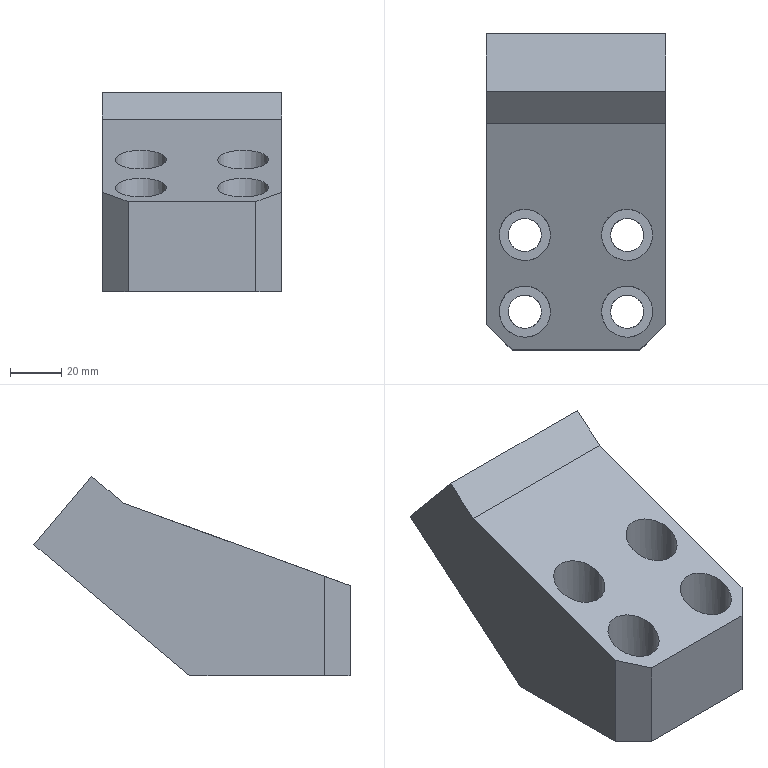Part | NX | features solid 2 | 1 solid | 22 faces | box 70 x 123.603 x 77.991 mm | volume 327595 mm3 | plane 14 | cylinder 8 | commonest cylinder face diameters 13 x4 20 x4
STEP:
#1=CARTESIAN_POINT('',(-535.,-473.5,-185.));
#2=VERTEX_POINT('',#1);
#3=CARTESIAN_POINT('',(-535.,-480.,-185.));
#4=DIRECTION('',(0.,0.,1.));
#5=DIRECTION('',(0.,1.,0.));
#6=AXIS2_PLACEMENT_3D('',#3,#4,#5);
#7=CIRCLE('',#6,6.5);
#8=EDGE_CURVE('',#2,#2,#7,.T.);
#9=ORIENTED_EDGE('',*,*,#8,.F.);
#10=EDGE_LOOP('',(#9));
#11=FACE_BOUND('',#10,.T.);
#12=CARTESIAN_POINT('',(-528.5,-480.,-165.));
#13=VERTEX_POINT('',#12);
#14=CARTESIAN_POINT('',(-535.,-480.,-165.));
#15=DIRECTION('',(0.,0.,1.));
#16=DIRECTION('',(1.,0.,0.));
#17=AXIS2_PLACEMENT_3D('',#14,#15,#16);
#18=CIRCLE('',#17,6.5);
#19=EDGE_CURVE('',#13,#13,#18,.F.);
#20=ORIENTED_EDGE('',*,*,#19,.F.);
#21=EDGE_LOOP('',(#20));
#22=FACE_BOUND('',#21,.T.);
#23=CARTESIAN_POINT('',(-535.,-480.,-135.));
#24=DIRECTION('',(0.,0.,-1.));
#25=DIRECTION('',(0.,-1.,0.));
#26=AXIS2_PLACEMENT_3D('',#23,#24,#25);
#27=CYLINDRICAL_SURFACE('',#26,6.5);
#28=ADVANCED_FACE('',(#11,#22),#27,.F.);
#29=CARTESIAN_POINT('',(-495.,-473.5,-185.));
#30=VERTEX_POINT('',#29);
#31=CARTESIAN_POINT('',(-495.,-480.,-185.));
#32=DIRECTION('',(0.,0.,1.));
#33=DIRECTION('',(0.,1.,0.));
#34=AXIS2_PLACEMENT_3D('',#31,#32,#33);
#35=CIRCLE('',#34,6.5);
#36=EDGE_CURVE('',#30,#30,#35,.T.);
#37=ORIENTED_EDGE('',*,*,#36,.F.);
#38=EDGE_LOOP('',(#37));
#39=FACE_BOUND('',#38,.T.);
#40=CARTESIAN_POINT('',(-488.5,-480.,-165.));
#41=VERTEX_POINT('',#40);
#42=CARTESIAN_POINT('',(-495.,-480.,-165.));
#43=DIRECTION('',(0.,0.,1.));
#44=DIRECTION('',(1.,0.,0.));
#45=AXIS2_PLACEMENT_3D('',#42,#43,#44);
#46=CIRCLE('',#45,6.5);
#47=EDGE_CURVE('',#41,#41,#46,.F.);
#48=ORIENTED_EDGE('',*,*,#47,.F.);
#49=EDGE_LOOP('',(#48));
#50=FACE_BOUND('',#49,.T.);
#51=CARTESIAN_POINT('',(-495.,-480.,-135.));
#52=DIRECTION('',(0.,0.,-1.));
#53=DIRECTION('',(0.,-1.,0.));
#54=AXIS2_PLACEMENT_3D('',#51,#52,#53);
#55=CYLINDRICAL_SURFACE('',#54,6.5);
#56=ADVANCED_FACE('',(#39,#50),#55,.F.);
#57=CARTESIAN_POINT('',(-495.,-503.5,-185.));
#58=VERTEX_POINT('',#57);
#59=CARTESIAN_POINT('',(-495.,-510.,-185.));
#60=DIRECTION('',(0.,0.,1.));
#61=DIRECTION('',(0.,1.,0.));
#62=AXIS2_PLACEMENT_3D('',#59,#60,#61);
#63=CIRCLE('',#62,6.5);
#64=EDGE_CURVE('',#58,#58,#63,.T.);
#65=ORIENTED_EDGE('',*,*,#64,.F.);
#66=EDGE_LOOP('',(#65));
#67=FACE_BOUND('',#66,.T.);
#68=CARTESIAN_POINT('',(-488.5,-510.,-165.));
#69=VERTEX_POINT('',#68);
#70=CARTESIAN_POINT('',(-495.,-510.,-165.));
#71=DIRECTION('',(0.,0.,1.));
#72=DIRECTION('',(1.,0.,0.));
#73=AXIS2_PLACEMENT_3D('',#70,#71,#72);
#74=CIRCLE('',#73,6.5);
#75=EDGE_CURVE('',#69,#69,#74,.F.);
#76=ORIENTED_EDGE('',*,*,#75,.F.);
#77=EDGE_LOOP('',(#76));
#78=FACE_BOUND('',#77,.T.);
#79=CARTESIAN_POINT('',(-495.,-510.,-135.));
#80=DIRECTION('',(0.,0.,-1.));
#81=DIRECTION('',(0.,-1.,0.));
#82=AXIS2_PLACEMENT_3D('',#79,#80,#81);
#83=CYLINDRICAL_SURFACE('',#82,6.5);
#84=ADVANCED_FACE('',(#67,#78),#83,.F.);
#85=CARTESIAN_POINT('',(-535.,-503.5,-185.));
#86=VERTEX_POINT('',#85);
#87=CARTESIAN_POINT('',(-535.,-510.,-185.));
#88=DIRECTION('',(0.,0.,1.));
#89=DIRECTION('',(0.,1.,0.));
#90=AXIS2_PLACEMENT_3D('',#87,#88,#89);
#91=CIRCLE('',#90,6.5);
#92=EDGE_CURVE('',#86,#86,#91,.T.);
#93=ORIENTED_EDGE('',*,*,#92,.F.);
#94=EDGE_LOOP('',(#93));
#95=FACE_BOUND('',#94,.T.);
#96=CARTESIAN_POINT('',(-528.5,-510.,-165.));
#97=VERTEX_POINT('',#96);
#98=CARTESIAN_POINT('',(-535.,-510.,-165.));
#99=DIRECTION('',(0.,0.,1.));
#100=DIRECTION('',(1.,0.,0.));
#101=AXIS2_PLACEMENT_3D('',#98,#99,#100);
#102=CIRCLE('',#101,6.5);
#103=EDGE_CURVE('',#97,#97,#102,.F.);
#104=ORIENTED_EDGE('',*,*,#103,.F.);
#105=EDGE_LOOP('',(#104));
#106=FACE_BOUND('',#105,.T.);
#107=CARTESIAN_POINT('',(-535.,-510.,-135.));
#108=DIRECTION('',(0.,0.,-1.));
#109=DIRECTION('',(0.,-1.,0.));
#110=AXIS2_PLACEMENT_3D('',#107,#108,#109);
#111=CYLINDRICAL_SURFACE('',#110,6.5);
#112=ADVANCED_FACE('',(#95,#106),#111,.F.);
#113=CARTESIAN_POINT('',(-540.,-525.,-185.));
#114=VERTEX_POINT('',#113);
#115=CARTESIAN_POINT('',(-490.,-525.,-185.));
#116=VERTEX_POINT('',#115);
#117=CARTESIAN_POINT('',(-535.,-525.,-185.));
#118=DIRECTION('',(-1.,0.,0.));
#119=VECTOR('',#118,1000.);
#120=LINE('',#117,#119);
#121=EDGE_CURVE('',#114,#116,#120,.F.);
#122=ORIENTED_EDGE('',*,*,#121,.T.);
#123=CARTESIAN_POINT('',(-490.,-525.,-149.753));
#124=VERTEX_POINT('',#123);
#125=CARTESIAN_POINT('',(-490.,-525.,-188.825));
#126=DIRECTION('',(0.,0.,-1.));
#127=VECTOR('',#126,1000.);
#128=LINE('',#125,#127);
#129=EDGE_CURVE('',#116,#124,#128,.F.);
#130=ORIENTED_EDGE('',*,*,#129,.T.);
#131=CARTESIAN_POINT('',(-540.,-525.,-149.753));
#132=VERTEX_POINT('',#131);
#133=CARTESIAN_POINT('',(-535.,-525.,-149.753));
#134=DIRECTION('',(1.,0.,0.));
#135=VECTOR('',#134,1000.);
#136=LINE('',#133,#135);
#137=EDGE_CURVE('',#124,#132,#136,.F.);
#138=ORIENTED_EDGE('',*,*,#137,.T.);
#139=CARTESIAN_POINT('',(-540.,-525.,-188.825));
#140=DIRECTION('',(0.,0.,1.));
#141=VECTOR('',#140,1000.);
#142=LINE('',#139,#141);
#143=EDGE_CURVE('',#132,#114,#142,.F.);
#144=ORIENTED_EDGE('',*,*,#143,.T.);
#145=EDGE_LOOP('',(#122,#130,#138,#144));
#146=FACE_BOUND('',#145,.T.);
#147=CARTESIAN_POINT('',(-535.,-525.,-188.825));
#148=DIRECTION('',(0.,-1.,0.));
#149=DIRECTION('',(1.,0.,0.));
#150=AXIS2_PLACEMENT_3D('',#147,#148,#149);
#151=PLANE('',#150);
#152=ADVANCED_FACE('',(#146),#151,.T.);
#153=CARTESIAN_POINT('',(-480.,-515.,-146.113));
#154=VERTEX_POINT('',#153);
#155=CARTESIAN_POINT('',(-480.,-515.,-185.));
#156=VERTEX_POINT('',#155);
#157=CARTESIAN_POINT('',(-480.,-515.,-188.825));
#158=DIRECTION('',(0.,0.,1.));
#159=VECTOR('',#158,1000.);
#160=LINE('',#157,#159);
#161=EDGE_CURVE('',#154,#156,#160,.F.);
#162=ORIENTED_EDGE('',*,*,#161,.T.);
#163=CARTESIAN_POINT('',(-480.,-462.389,-185.));
#164=VERTEX_POINT('',#163);
#165=CARTESIAN_POINT('',(-480.,-492.776,-185.));
#166=DIRECTION('',(0.,-1.,0.));
#167=VECTOR('',#166,1000.);
#168=LINE('',#165,#167);
#169=EDGE_CURVE('',#156,#164,#168,.F.);
#170=ORIENTED_EDGE('',*,*,#169,.T.);
#171=CARTESIAN_POINT('',(-480.,-401.397,-133.821));
#172=VERTEX_POINT('',#171);
#173=CARTESIAN_POINT('',(-480.,-482.104,-201.543));
#174=DIRECTION('',(0.,-0.766,-0.6428));
#175=VECTOR('',#174,1000.);
#176=LINE('',#173,#175);
#177=EDGE_CURVE('',#164,#172,#176,.F.);
#178=ORIENTED_EDGE('',*,*,#177,.T.);
#179=CARTESIAN_POINT('',(-480.,-423.894,-107.009));
#180=VERTEX_POINT('',#179);
#181=CARTESIAN_POINT('',(-480.,-406.76,-127.429));
#182=DIRECTION('',(0.,0.6428,-0.766));
#183=VECTOR('',#182,1000.);
#184=LINE('',#181,#183);
#185=EDGE_CURVE('',#180,#172,#184,.T.);
#186=ORIENTED_EDGE('',*,*,#185,.F.);
#187=CARTESIAN_POINT('',(-480.,-436.404,-117.506));
#188=VERTEX_POINT('',#187);
#189=CARTESIAN_POINT('',(-480.,-435.385,-116.651));
#190=DIRECTION('',(0.,-0.766,-0.6428));
#191=VECTOR('',#190,1000.);
#192=LINE('',#189,#191);
#193=EDGE_CURVE('',#188,#180,#192,.F.);
#194=ORIENTED_EDGE('',*,*,#193,.F.);
#195=CARTESIAN_POINT('',(-480.,-509.103,-143.966));
#196=DIRECTION('',(0.,0.9397,0.342));
#197=VECTOR('',#196,1000.);
#198=LINE('',#195,#197);
#199=EDGE_CURVE('',#154,#188,#198,.T.);
#200=ORIENTED_EDGE('',*,*,#199,.F.);
#201=EDGE_LOOP('',(#162,#170,#178,#186,#194,#200));
#202=FACE_BOUND('',#201,.T.);
#203=CARTESIAN_POINT('',(-480.,-492.776,-188.825));
#204=DIRECTION('',(1.,0.,0.));
#205=DIRECTION('',(0.,1.,0.));
#206=AXIS2_PLACEMENT_3D('',#203,#204,#205);
#207=PLANE('',#206);
#208=ADVANCED_FACE('',(#202),#207,.T.);
#209=CARTESIAN_POINT('',(-550.,-436.404,-117.506));
#210=VERTEX_POINT('',#209);
#211=CARTESIAN_POINT('',(-550.,-423.894,-107.009));
#212=VERTEX_POINT('',#211);
#213=CARTESIAN_POINT('',(-550.,-504.602,-174.731));
#214=DIRECTION('',(0.,0.766,0.6428));
#215=VECTOR('',#214,1000.);
#216=LINE('',#213,#215);
#217=EDGE_CURVE('',#210,#212,#216,.T.);
#218=ORIENTED_EDGE('',*,*,#217,.T.);
#219=CARTESIAN_POINT('',(-550.,-401.397,-133.821));
#220=VERTEX_POINT('',#219);
#221=CARTESIAN_POINT('',(-550.,-406.76,-127.429));
#222=DIRECTION('',(0.,-0.6428,0.766));
#223=VECTOR('',#222,1000.);
#224=LINE('',#221,#223);
#225=EDGE_CURVE('',#220,#212,#224,.T.);
#226=ORIENTED_EDGE('',*,*,#225,.F.);
#227=CARTESIAN_POINT('',(-550.,-462.389,-185.));
#228=VERTEX_POINT('',#227);
#229=CARTESIAN_POINT('',(-550.,-412.887,-143.463));
#230=DIRECTION('',(0.,0.766,0.6428));
#231=VECTOR('',#230,1000.);
#232=LINE('',#229,#231);
#233=EDGE_CURVE('',#228,#220,#232,.T.);
#234=ORIENTED_EDGE('',*,*,#233,.F.);
#235=CARTESIAN_POINT('',(-550.,-515.,-185.));
#236=VERTEX_POINT('',#235);
#237=CARTESIAN_POINT('',(-550.,-492.776,-185.));
#238=DIRECTION('',(0.,-1.,0.));
#239=VECTOR('',#238,1000.);
#240=LINE('',#237,#239);
#241=EDGE_CURVE('',#228,#236,#240,.T.);
#242=ORIENTED_EDGE('',*,*,#241,.T.);
#243=CARTESIAN_POINT('',(-550.,-515.,-146.113));
#244=VERTEX_POINT('',#243);
#245=CARTESIAN_POINT('',(-550.,-515.,-188.825));
#246=DIRECTION('',(0.,0.,1.));
#247=VECTOR('',#246,1000.);
#248=LINE('',#245,#247);
#249=EDGE_CURVE('',#236,#244,#248,.T.);
#250=ORIENTED_EDGE('',*,*,#249,.T.);
#251=CARTESIAN_POINT('',(-550.,-509.103,-143.966));
#252=DIRECTION('',(0.,0.9397,0.342));
#253=VECTOR('',#252,1000.);
#254=LINE('',#251,#253);
#255=EDGE_CURVE('',#210,#244,#254,.F.);
#256=ORIENTED_EDGE('',*,*,#255,.F.);
#257=EDGE_LOOP('',(#218,#226,#234,#242,#250,#256));
#258=FACE_BOUND('',#257,.T.);
#259=CARTESIAN_POINT('',(-550.,-492.776,-188.825));
#260=DIRECTION('',(1.,0.,0.));
#261=DIRECTION('',(0.,1.,0.));
#262=AXIS2_PLACEMENT_3D('',#259,#260,#261);
#263=PLANE('',#262);
#264=ADVANCED_FACE('',(#258),#263,.F.);
#265=ORIENTED_EDGE('',*,*,#64,.T.);
#266=EDGE_LOOP('',(#265));
#267=FACE_BOUND('',#266,.T.);
#268=ORIENTED_EDGE('',*,*,#92,.T.);
#269=EDGE_LOOP('',(#268));
#270=FACE_BOUND('',#269,.T.);
#271=ORIENTED_EDGE('',*,*,#169,.F.);
#272=CARTESIAN_POINT('',(-480.,-515.,-185.));
#273=DIRECTION('',(0.7071,0.7071,0.));
#274=VECTOR('',#273,1000.);
#275=LINE('',#272,#274);
#276=EDGE_CURVE('',#156,#116,#275,.F.);
#277=ORIENTED_EDGE('',*,*,#276,.T.);
#278=ORIENTED_EDGE('',*,*,#121,.F.);
#279=CARTESIAN_POINT('',(-540.,-525.,-185.));
#280=DIRECTION('',(-0.7071,0.7071,0.));
#281=VECTOR('',#280,1000.);
#282=LINE('',#279,#281);
#283=EDGE_CURVE('',#114,#236,#282,.T.);
#284=ORIENTED_EDGE('',*,*,#283,.T.);
#285=ORIENTED_EDGE('',*,*,#241,.F.);
#286=CARTESIAN_POINT('',(-515.,-462.389,-185.));
#287=DIRECTION('',(-1.,0.,0.));
#288=VECTOR('',#287,1000.);
#289=LINE('',#286,#288);
#290=EDGE_CURVE('',#164,#228,#289,.T.);
#291=ORIENTED_EDGE('',*,*,#290,.F.);
#292=EDGE_LOOP('',(#271,#277,#278,#284,#285,#291));
#293=FACE_BOUND('',#292,.T.);
#294=ORIENTED_EDGE('',*,*,#36,.T.);
#295=EDGE_LOOP('',(#294));
#296=FACE_BOUND('',#295,.T.);
#297=ORIENTED_EDGE('',*,*,#8,.T.);
#298=EDGE_LOOP('',(#297));
#299=FACE_BOUND('',#298,.T.);
#300=CARTESIAN_POINT('',(-203.,-82.,-185.));
#301=DIRECTION('',(0.,0.,1.));
#302=DIRECTION('',(0.,1.,0.));
#303=AXIS2_PLACEMENT_3D('',#300,#301,#302);
#304=PLANE('',#303);
#305=ADVANCED_FACE('',(#267,#270,#293,#296,#299),#304,.F.);
#306=ORIENTED_EDGE('',*,*,#129,.F.);
#307=ORIENTED_EDGE('',*,*,#276,.F.);
#308=ORIENTED_EDGE('',*,*,#161,.F.);
#309=CARTESIAN_POINT('',(-469.616,-504.616,-142.333));
#310=DIRECTION('',(0.6848,0.6848,0.2492));
#311=VECTOR('',#310,1000.);
#312=LINE('',#309,#311);
#313=EDGE_CURVE('',#124,#154,#312,.T.);
#314=ORIENTED_EDGE('',*,*,#313,.F.);
#315=EDGE_LOOP('',(#306,#307,#308,#314));
#316=FACE_BOUND('',#315,.T.);
#317=CARTESIAN_POINT('',(-480.,-515.,-188.825));
#318=DIRECTION('',(-0.7071,0.7071,0.));
#319=DIRECTION('',(-0.7071,-0.7071,0.));
#320=AXIS2_PLACEMENT_3D('',#317,#318,#319);
#321=PLANE('',#320);
#322=ADVANCED_FACE('',(#316),#321,.F.);
#323=CARTESIAN_POINT('',(-533.331,-531.669,-152.18));
#324=DIRECTION('',(0.6848,-0.6848,-0.2492));
#325=VECTOR('',#324,1000.);
#326=LINE('',#323,#325);
#327=EDGE_CURVE('',#132,#244,#326,.F.);
#328=ORIENTED_EDGE('',*,*,#327,.T.);
#329=ORIENTED_EDGE('',*,*,#249,.F.);
#330=ORIENTED_EDGE('',*,*,#283,.F.);
#331=ORIENTED_EDGE('',*,*,#143,.F.);
#332=EDGE_LOOP('',(#328,#329,#330,#331));
#333=FACE_BOUND('',#332,.T.);
#334=CARTESIAN_POINT('',(-540.,-525.,-188.825));
#335=DIRECTION('',(-0.7071,-0.7071,0.));
#336=DIRECTION('',(0.7071,-0.7071,0.));
#337=AXIS2_PLACEMENT_3D('',#334,#335,#336);
#338=PLANE('',#337);
#339=ADVANCED_FACE('',(#333),#338,.T.);
#340=CARTESIAN_POINT('',(-525.,-510.,-165.));
#341=VERTEX_POINT('',#340);
#342=CARTESIAN_POINT('',(-535.,-510.,-165.));
#343=DIRECTION('',(0.,0.,1.));
#344=DIRECTION('',(1.,0.,0.));
#345=AXIS2_PLACEMENT_3D('',#342,#343,#344);
#346=CIRCLE('',#345,10.);
#347=EDGE_CURVE('',#341,#341,#346,.T.);
#348=ORIENTED_EDGE('',*,*,#347,.T.);
#349=EDGE_LOOP('',(#348));
#350=FACE_BOUND('',#349,.T.);
#351=ORIENTED_EDGE('',*,*,#103,.T.);
#352=EDGE_LOOP('',(#351));
#353=FACE_BOUND('',#352,.T.);
#354=CARTESIAN_POINT('',(-535.,-510.,-165.));
#355=DIRECTION('',(0.,0.,1.));
#356=DIRECTION('',(0.,1.,0.));
#357=AXIS2_PLACEMENT_3D('',#354,#355,#356);
#358=PLANE('',#357);
#359=ADVANCED_FACE('',(#350,#353),#358,.T.);
#360=CARTESIAN_POINT('',(-535.,-520.,-147.933));
#361=VERTEX_POINT('',#360);
#362=CARTESIAN_POINT('',(-535.,-510.,-144.293));
#363=DIRECTION('',(0.,0.342,-0.9397));
#364=DIRECTION('',(0.,-0.9397,-0.342));
#365=AXIS2_PLACEMENT_3D('',#362,#363,#364);
#366=ELLIPSE('',#365,10.642,10.);
#367=EDGE_CURVE('',#361,#361,#366,.T.);
#368=ORIENTED_EDGE('',*,*,#367,.F.);
#369=EDGE_LOOP('',(#368));
#370=FACE_BOUND('',#369,.T.);
#371=ORIENTED_EDGE('',*,*,#347,.F.);
#372=EDGE_LOOP('',(#371));
#373=FACE_BOUND('',#372,.T.);
#374=CARTESIAN_POINT('',(-535.,-510.,15.));
#375=DIRECTION('',(0.,0.,-1.));
#376=DIRECTION('',(0.,-1.,0.));
#377=AXIS2_PLACEMENT_3D('',#374,#375,#376);
#378=CYLINDRICAL_SURFACE('',#377,10.);
#379=ADVANCED_FACE('',(#370,#373),#378,.F.);
#380=CARTESIAN_POINT('',(-485.,-510.,-165.));
#381=VERTEX_POINT('',#380);
#382=CARTESIAN_POINT('',(-495.,-510.,-165.));
#383=DIRECTION('',(0.,0.,1.));
#384=DIRECTION('',(1.,0.,0.));
#385=AXIS2_PLACEMENT_3D('',#382,#383,#384);
#386=CIRCLE('',#385,10.);
#387=EDGE_CURVE('',#381,#381,#386,.T.);
#388=ORIENTED_EDGE('',*,*,#387,.T.);
#389=EDGE_LOOP('',(#388));
#390=FACE_BOUND('',#389,.T.);
#391=ORIENTED_EDGE('',*,*,#75,.T.);
#392=EDGE_LOOP('',(#391));
#393=FACE_BOUND('',#392,.T.);
#394=CARTESIAN_POINT('',(-495.,-510.,-165.));
#395=DIRECTION('',(0.,0.,1.));
#396=DIRECTION('',(0.,1.,0.));
#397=AXIS2_PLACEMENT_3D('',#394,#395,#396);
#398=PLANE('',#397);
#399=ADVANCED_FACE('',(#390,#393),#398,.T.);
#400=CARTESIAN_POINT('',(-495.,-520.,-147.933));
#401=VERTEX_POINT('',#400);
#402=CARTESIAN_POINT('',(-495.,-510.,-144.293));
#403=DIRECTION('',(0.,0.342,-0.9397));
#404=DIRECTION('',(0.,-0.9397,-0.342));
#405=AXIS2_PLACEMENT_3D('',#402,#403,#404);
#406=ELLIPSE('',#405,10.642,10.);
#407=EDGE_CURVE('',#401,#401,#406,.T.);
#408=ORIENTED_EDGE('',*,*,#407,.F.);
#409=EDGE_LOOP('',(#408));
#410=FACE_BOUND('',#409,.T.);
#411=ORIENTED_EDGE('',*,*,#387,.F.);
#412=EDGE_LOOP('',(#411));
#413=FACE_BOUND('',#412,.T.);
#414=CARTESIAN_POINT('',(-495.,-510.,15.));
#415=DIRECTION('',(0.,0.,-1.));
#416=DIRECTION('',(0.,-1.,0.));
#417=AXIS2_PLACEMENT_3D('',#414,#415,#416);
#418=CYLINDRICAL_SURFACE('',#417,10.);
#419=ADVANCED_FACE('',(#410,#413),#418,.F.);
#420=CARTESIAN_POINT('',(-485.,-480.,-165.));
#421=VERTEX_POINT('',#420);
#422=CARTESIAN_POINT('',(-495.,-480.,-165.));
#423=DIRECTION('',(0.,0.,1.));
#424=DIRECTION('',(1.,0.,0.));
#425=AXIS2_PLACEMENT_3D('',#422,#423,#424);
#426=CIRCLE('',#425,10.);
#427=EDGE_CURVE('',#421,#421,#426,.T.);
#428=ORIENTED_EDGE('',*,*,#427,.T.);
#429=EDGE_LOOP('',(#428));
#430=FACE_BOUND('',#429,.T.);
#431=ORIENTED_EDGE('',*,*,#47,.T.);
#432=EDGE_LOOP('',(#431));
#433=FACE_BOUND('',#432,.T.);
#434=CARTESIAN_POINT('',(-495.,-480.,-165.));
#435=DIRECTION('',(0.,0.,1.));
#436=DIRECTION('',(0.,1.,0.));
#437=AXIS2_PLACEMENT_3D('',#434,#435,#436);
#438=PLANE('',#437);
#439=ADVANCED_FACE('',(#430,#433),#438,.T.);
#440=CARTESIAN_POINT('',(-495.,-490.,-137.014));
#441=VERTEX_POINT('',#440);
#442=CARTESIAN_POINT('',(-495.,-480.,-133.374));
#443=DIRECTION('',(0.,0.342,-0.9397));
#444=DIRECTION('',(0.,-0.9397,-0.342));
#445=AXIS2_PLACEMENT_3D('',#442,#443,#444);
#446=ELLIPSE('',#445,10.642,10.);
#447=EDGE_CURVE('',#441,#441,#446,.T.);
#448=ORIENTED_EDGE('',*,*,#447,.F.);
#449=EDGE_LOOP('',(#448));
#450=FACE_BOUND('',#449,.T.);
#451=ORIENTED_EDGE('',*,*,#427,.F.);
#452=EDGE_LOOP('',(#451));
#453=FACE_BOUND('',#452,.T.);
#454=CARTESIAN_POINT('',(-495.,-480.,15.));
#455=DIRECTION('',(0.,0.,-1.));
#456=DIRECTION('',(0.,-1.,0.));
#457=AXIS2_PLACEMENT_3D('',#454,#455,#456);
#458=CYLINDRICAL_SURFACE('',#457,10.);
#459=ADVANCED_FACE('',(#450,#453),#458,.F.);
#460=CARTESIAN_POINT('',(-525.,-480.,-165.));
#461=VERTEX_POINT('',#460);
#462=CARTESIAN_POINT('',(-535.,-480.,-165.));
#463=DIRECTION('',(0.,0.,1.));
#464=DIRECTION('',(1.,0.,0.));
#465=AXIS2_PLACEMENT_3D('',#462,#463,#464);
#466=CIRCLE('',#465,10.);
#467=EDGE_CURVE('',#461,#461,#466,.T.);
#468=ORIENTED_EDGE('',*,*,#467,.T.);
#469=EDGE_LOOP('',(#468));
#470=FACE_BOUND('',#469,.T.);
#471=ORIENTED_EDGE('',*,*,#19,.T.);
#472=EDGE_LOOP('',(#471));
#473=FACE_BOUND('',#472,.T.);
#474=CARTESIAN_POINT('',(-535.,-480.,-165.));
#475=DIRECTION('',(0.,0.,1.));
#476=DIRECTION('',(0.,1.,0.));
#477=AXIS2_PLACEMENT_3D('',#474,#475,#476);
#478=PLANE('',#477);
#479=ADVANCED_FACE('',(#470,#473),#478,.T.);
#480=CARTESIAN_POINT('',(-535.,-490.,-137.014));
#481=VERTEX_POINT('',#480);
#482=CARTESIAN_POINT('',(-535.,-480.,-133.374));
#483=DIRECTION('',(0.,0.342,-0.9397));
#484=DIRECTION('',(0.,-0.9397,-0.342));
#485=AXIS2_PLACEMENT_3D('',#482,#483,#484);
#486=ELLIPSE('',#485,10.642,10.);
#487=EDGE_CURVE('',#481,#481,#486,.T.);
#488=ORIENTED_EDGE('',*,*,#487,.F.);
#489=EDGE_LOOP('',(#488));
#490=FACE_BOUND('',#489,.T.);
#491=ORIENTED_EDGE('',*,*,#467,.F.);
#492=EDGE_LOOP('',(#491));
#493=FACE_BOUND('',#492,.T.);
#494=CARTESIAN_POINT('',(-535.,-480.,15.));
#495=DIRECTION('',(0.,0.,-1.));
#496=DIRECTION('',(0.,-1.,0.));
#497=AXIS2_PLACEMENT_3D('',#494,#495,#496);
#498=CYLINDRICAL_SURFACE('',#497,10.);
#499=ADVANCED_FACE('',(#490,#493),#498,.F.);
#500=ORIENTED_EDGE('',*,*,#290,.T.);
#501=ORIENTED_EDGE('',*,*,#233,.T.);
#502=CARTESIAN_POINT('',(-515.,-401.397,-133.821));
#503=DIRECTION('',(-1.,0.,0.));
#504=VECTOR('',#503,1000.);
#505=LINE('',#502,#504);
#506=EDGE_CURVE('',#172,#220,#505,.T.);
#507=ORIENTED_EDGE('',*,*,#506,.F.);
#508=ORIENTED_EDGE('',*,*,#177,.F.);
#509=EDGE_LOOP('',(#500,#501,#507,#508));
#510=FACE_BOUND('',#509,.T.);
#511=CARTESIAN_POINT('',(-515.,-412.887,-143.463));
#512=DIRECTION('',(0.,0.6428,-0.766));
#513=DIRECTION('',(0.,0.766,0.6428));
#514=AXIS2_PLACEMENT_3D('',#511,#512,#513);
#515=PLANE('',#514);
#516=ADVANCED_FACE('',(#510),#515,.T.);
#517=ORIENTED_EDGE('',*,*,#193,.T.);
#518=CARTESIAN_POINT('',(-515.,-423.894,-107.009));
#519=DIRECTION('',(1.,0.,0.));
#520=VECTOR('',#519,1000.);
#521=LINE('',#518,#520);
#522=EDGE_CURVE('',#212,#180,#521,.T.);
#523=ORIENTED_EDGE('',*,*,#522,.F.);
#524=ORIENTED_EDGE('',*,*,#217,.F.);
#525=CARTESIAN_POINT('',(-515.,-436.404,-117.506));
#526=DIRECTION('',(1.,0.,0.));
#527=VECTOR('',#526,1000.);
#528=LINE('',#525,#527);
#529=EDGE_CURVE('',#188,#210,#528,.F.);
#530=ORIENTED_EDGE('',*,*,#529,.F.);
#531=EDGE_LOOP('',(#517,#523,#524,#530));
#532=FACE_BOUND('',#531,.T.);
#533=CARTESIAN_POINT('',(-515.,-435.385,-116.651));
#534=DIRECTION('',(0.,-0.6428,0.766));
#535=DIRECTION('',(0.,-0.766,-0.6428));
#536=AXIS2_PLACEMENT_3D('',#533,#534,#535);
#537=PLANE('',#536);
#538=ADVANCED_FACE('',(#532),#537,.T.);
#539=ORIENTED_EDGE('',*,*,#522,.T.);
#540=ORIENTED_EDGE('',*,*,#185,.T.);
#541=ORIENTED_EDGE('',*,*,#506,.T.);
#542=ORIENTED_EDGE('',*,*,#225,.T.);
#543=EDGE_LOOP('',(#539,#540,#541,#542));
#544=FACE_BOUND('',#543,.T.);
#545=CARTESIAN_POINT('',(-515.,-406.76,-127.429));
#546=DIRECTION('',(0.,0.766,0.6428));
#547=DIRECTION('',(-1.,0.,0.));
#548=AXIS2_PLACEMENT_3D('',#545,#546,#547);
#549=PLANE('',#548);
#550=ADVANCED_FACE('',(#544),#549,.T.);
#551=ORIENTED_EDGE('',*,*,#313,.T.);
#552=ORIENTED_EDGE('',*,*,#199,.T.);
#553=ORIENTED_EDGE('',*,*,#529,.T.);
#554=ORIENTED_EDGE('',*,*,#255,.T.);
#555=ORIENTED_EDGE('',*,*,#327,.F.);
#556=ORIENTED_EDGE('',*,*,#137,.F.);
#557=EDGE_LOOP('',(#551,#552,#553,#554,#555,#556));
#558=FACE_BOUND('',#557,.T.);
#559=ORIENTED_EDGE('',*,*,#407,.T.);
#560=EDGE_LOOP('',(#559));
#561=FACE_BOUND('',#560,.T.);
#562=ORIENTED_EDGE('',*,*,#367,.T.);
#563=EDGE_LOOP('',(#562));
#564=FACE_BOUND('',#563,.T.);
#565=ORIENTED_EDGE('',*,*,#447,.T.);
#566=EDGE_LOOP('',(#565));
#567=FACE_BOUND('',#566,.T.);
#568=ORIENTED_EDGE('',*,*,#487,.T.);
#569=EDGE_LOOP('',(#568));
#570=FACE_BOUND('',#569,.T.);
#571=CARTESIAN_POINT('',(-515.,-464.541,-127.747));
#572=DIRECTION('',(0.,-0.342,0.9397));
#573=DIRECTION('',(0.,-0.9397,-0.342));
#574=AXIS2_PLACEMENT_3D('',#571,#572,#573);
#575=PLANE('',#574);
#576=ADVANCED_FACE('',(#558,#561,#564,#567,#570),#575,.T.);
#577=CLOSED_SHELL('',(#28,#56,#84,#112,#152,#208,#264,#305,#322,#339,#359,#379,#399,#419,#439,#459,#479,#499,#516,#538,#550,#576));
#578=MANIFOLD_SOLID_BREP('',#577);
#579=(LENGTH_UNIT()NAMED_UNIT(*)SI_UNIT(.MILLI.,.METRE.));
#580=UNCERTAINTY_MEASURE_WITH_UNIT(LENGTH_MEASURE(0.00001),#579,'','');
#581=(NAMED_UNIT(*)PLANE_ANGLE_UNIT()SI_UNIT($,.RADIAN.));
#582=(NAMED_UNIT(*)SI_UNIT($,.STERADIAN.)SOLID_ANGLE_UNIT());
#583=(GEOMETRIC_REPRESENTATION_CONTEXT(3)GLOBAL_UNCERTAINTY_ASSIGNED_CONTEXT((#580))GLOBAL_UNIT_ASSIGNED_CONTEXT((#579,#581,#582))REPRESENTATION_CONTEXT('',''));
#584=ADVANCED_BREP_SHAPE_REPRESENTATION('',(#578),#583);